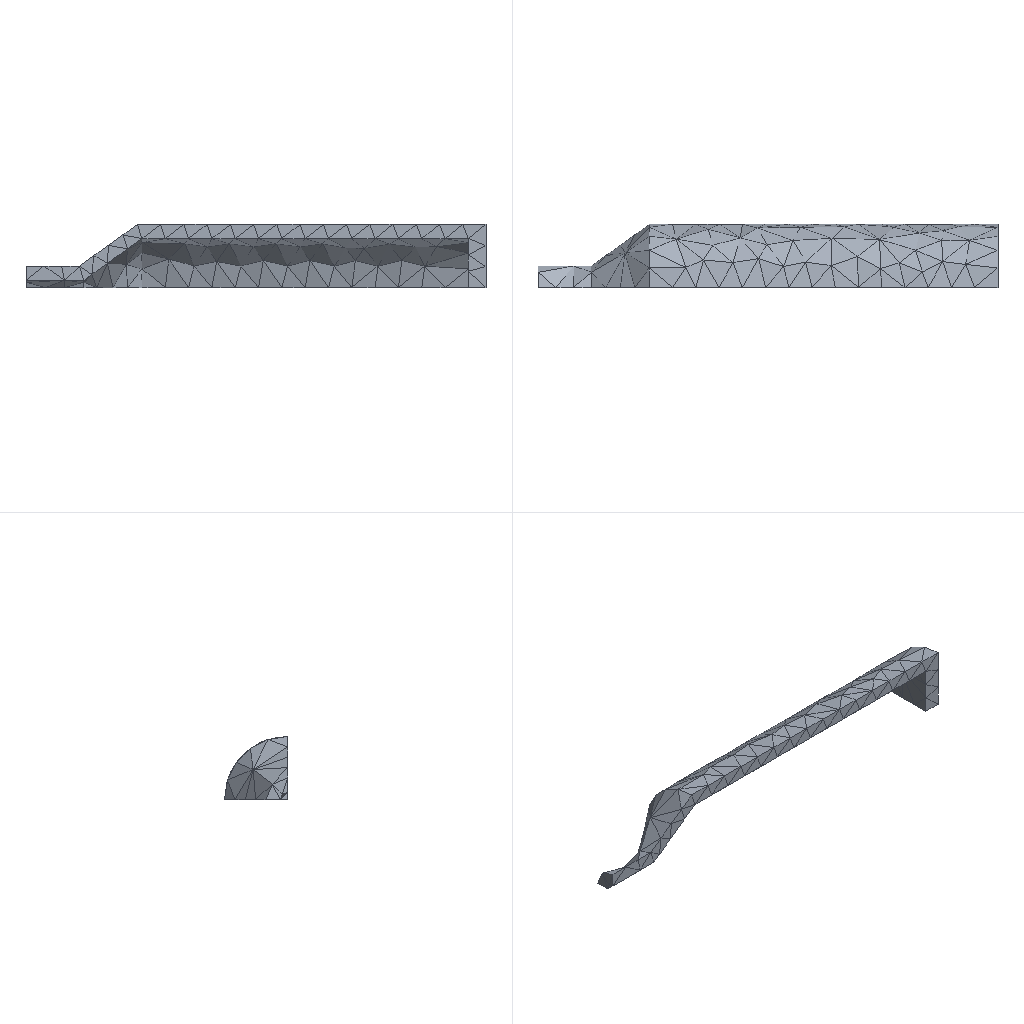Simulation study | ansys workbench
Ansys APDL input file, long lists of numbers shortened:
/batch
/config,noeldb,1     ! force off writing results to database
*get,_wallstrt,active,,time,wall
! ANSYS input file written by Workbench version 2022 R1
! File used for geometry attach:
/title,wbnew--____ (C5)
! ****** Begin Custom Load Command Snippet ******
/COM, ACT Extensions:
/COM,     LSDYNA, 2021.1
/COM,
! ****** End   Custom Load Command Snippet ******
*DIM,_wb_ProjectScratch_dir,string,248
_wb_ProjectScratch_dir(1) = ''
*DIM,_wb_SolverFiles_dir,string,248
_wb_SolverFiles_dir(1) = ''
*DIM,_wb_userfiles_dir,string,248
_wb_userfiles_dir(1) = ''
/com,--- Data in consistent NMM units. See Solving Units in the help system for more information.
/units,MPA
/nopr
/wb,file,start              !  signify a WB generated input file
/prep7
! Turn off shape checking because checks already performed inside WB mesher.
! See help system for more information.
SHPP,OFF,,NOWARN
/nolist
etcon,set             ! allow ANSYS to choose best KEYOP's for 180x elements, resets any applicable keyopt to MAPDL defaults
/com,*********** Nodes for the whole assembly ***********
nblock,3,,975
(1i9,3e20.9e3)
        1     1.305000000E+03     0.000000000E+00     0.000000000E+00
! (886 more lines like these left out)
-1
/wb,elem,start            !  set before creation of elements
/com,*********** Elements for Body 1 "__3-FreeParts|__-__3" ***********
et,1,187
eblock,19,solid,,368
(19i9)
        1        1        1        1        0        0        0        0       10        0        1       25       94       93      131      303      594      302      304
! (735 more lines like these left out)
-1
/wb,elem,end               !  done creating elements
/com,*********** Send User Defined Coordinate System(s) ***********
csys,0
toffst,273.15,  ! Temperature offset from absolute zero
/com,*********** Set Reference Temperature ***********
tref,22.
/wb,mat,start              !  starting to send materials
/com,*********** Send Materials ***********
Temperature = 'TEMP' ! Temperature
MP,DENS,1,7.85e-09,	! tonne mm^-3
MP,ALPX,1,1.2e-05,	! C^-1
MP,C,1,434000000,	! mm^2 s^-2 C^-1
MP,KXX,1,60.5,	! tonne mm s^-3 C^-1
MP,RSVX,1,0.00017,	! ohm mm
MP,EX,1,200000,	! tonne s^-2 mm^-1
MP,NUXY,1,0.3,
MP,MURX,1,10000,
/wb,mat,end                !  done sending materials
!************************* Model Summary ********************
!__3-FreeParts|__-__3,	结构钢,	matid,	1
!************************* End Model Summary ********************
! get the diagonal of the bounding box. Needed later for other things
*get,_xmin,node,,mnloc,x
*get,_ymin,node,,mnloc,y
*get,_zmin,node,,mnloc,z
*get,_xmax,node,,mxloc,x
*get,_ymax,node,,mxloc,y
*get,_zmax,node,,mxloc,z
_ASMDIAG=(_xmax-_xmin)*(_xmax-_xmin)+(_ymax-_ymin)*(_ymax-_ymin)+(_zmax-_zmin)*(_zmax-_zmin)
_ASMDIAG=SQRT(_ASMDIAG)
/wb,contact,start          !  starting to send contact
/wb,contact,end            !  done creating contacts
/golist
/wb,load,start             !  starting to send loads
/com,*********** Fixed Supports ***********
CMBLOCK,_FIXEDSU,NODE,       34
(8i10)
         1         2         3         4         5         6         7         8
         9        10        11       174       175       176       180       181
       184       185       189       190       194       195       196       199
       200       204       207       208       213       214       219       220
       224       230
cmsel,s,_FIXEDSU
d,all,all
nsel,all
/com,*********** Define Pressure Using Surface Effect Elements "__" ***********
et,2,154
eblock,10,,,100
(15i9)
      713        2        2        2        0        2        8       45       45      181      209       45      182
! (99 more lines like these left out)
-1
esel,s,type,,2
keyop,2,7,0                ! Use deformed area for application of load
esel,all
/com,*********** Define Pressure Using Surface Effect Elements "__ 2" ***********
et,3,154
eblock,10,,,82
(15i9)
      813        3        3        3        0       99       75      121      121      525      528      121      625
! (81 more lines like these left out)
-1
esel,s,type,,3
keyop,3,7,0                ! Use deformed area for application of load
esel,all
esel,all
/gst,on,on
fini
*get,_numnode,node,0,count
*get,_numelem,elem,0,count
*get, _MAXELEMNUM, elem, 0, NUM, MAX
*get, _MAXNODENUM, node, 0, NUM, MAX
*get, _MAXELEMTYPE, etyp, 0, NUM, MAX
*get, _MAXREALCONST, real, 0, NUM, MAX
/go
/wb,load,end               !  done creating loads
/com,--- Number of total nodes = %_numnode%
/com,--- Number of contact elements = 182
/com,--- Number of spring elements = 0
/com,--- Number of bearing elements = 0
/com,--- Number of solid elements = 368
/com,--- Number of condensed parts = 0
/com,--- Number of total elements = %_numelem%
*get,_wallbsol,active,,time,wall
/com,****************************************************************************
/com,*************************    SOLUTION       ********************************
/com,****************************************************************************
/solu
antype,0                   ! static analysis
_thickRatio=  0     ! Ratio of thick parts in the model
eqsl,sparse,,,,,1
cntr,print,1               ! print out contact info and also make no initial contact an error
dmpoption,emat,no             ! Don't combine emat file for DANSYS
dmpoption,esav,no             ! Don't combine esav file for DANSYS
nldiag,cont,iter           ! print out contact info each equilibrium iteration
rescontrol,,none                 ! Do not keep any restart files
/com,****************************************************
/com,******************* SOLVE FOR LS 1 OF 1 ****************
esel,s,type,,2
nsle
sf,all,pres,20.
esel,s,type,,3
nsle
sf,all,pres,60.
nsel,all
esel,all
esel,all
/nopr
/gopr
nsub,1,1,1
time,1.
outres,erase
outres,all,none
outres,nsol,all,
outres,rsol,all
outres,eangl,all
outres,etmp,all
outres,veng,all
outres,strs,all,
outres,epel,all,
outres,eppl,all,
outres,cont,all,
! *********** WB SOLVE COMMAND ***********
! check interactive state
*get,ANSINTER_,active,,int
*if,ANSINTER_,ne,0,then
/eof
*endif
solve
/com *************** Write FE CONNECTORS *********
CEWRITE,file,ce,,INTE
/com,****************************************************
/com,*************** FINISHED SOLVE FOR LS 1 *************
*get,_wallasol,active,,time,wall
/nopr
*get,_numnode,node,0,count
*get,_numelem,elem,0,count
*get, _MAXELEMNUM, elem, 0, NUM, MAX
*get, _MAXNODENUM, node, 0, NUM, MAX,,,INTERNAL
*get, _MAXELEMTYPE, etyp, 0, NUM, MAX
*get, _MAXREALCONST, real, 0, NUM, MAX
/gopr
/post1
xmlo,ENCODING,ISO-8859-1
xmlo,parm
/xml,parm,xml
fini
/gopr
*get,_walldone,active,,time,wall
_preptime=(_wallbsol-_wallstrt)*3600
_solvtime=(_wallasol-_wallbsol)*3600
_posttime=(_walldone-_wallasol)*3600
_totaltim=(_walldone-_wallstrt)*3600
*get,_dlbratio,active,0,solu,dlbr
*get,_combtime,active,0,solu,comb
*get,_ssmode,active,0,solu,ssmm
*get,_ndofs,active,0,solu,ndof
*get,_sol_end_time,active,0,set,time
*if,_sol_end_time,eq,1.,then
/fclean				!clean distributed files
*endif
/com,--- Total number of nodes = %_numnode%
/com,--- Total number of elements = %_numelem%
/com,--- Element load balance ratio = %_dlbratio%
/com,--- Time to combine distributed files = %_combtime%
/com,--- Sparse memory mode = %_ssmode%
/com,--- Number of DOF = %_ndofs%
/wb,file,end               ! done with WB generated input